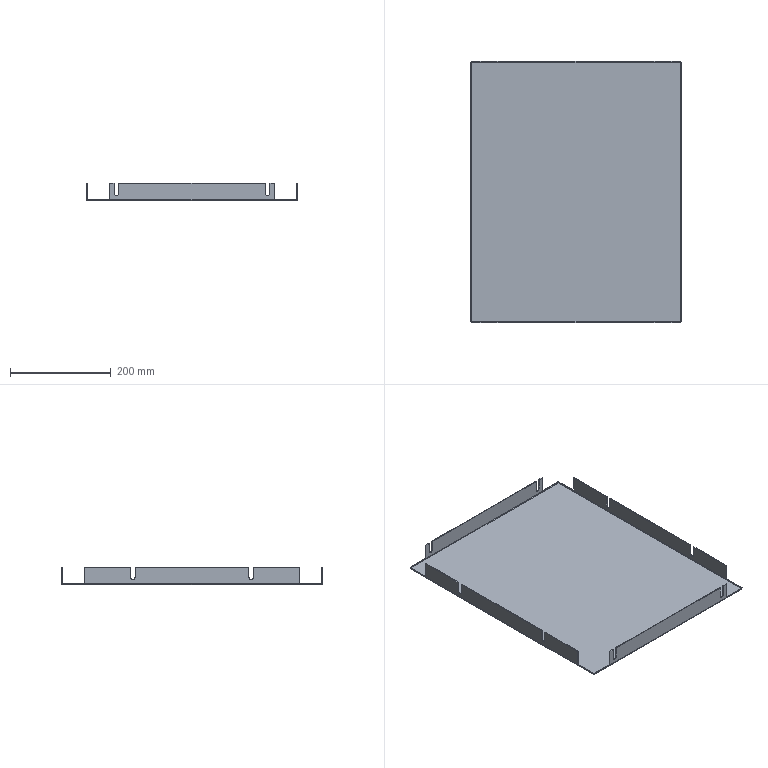Part | SolidWorks | features BaseBody 1 | 1 solid | 90 faces | box 418 x 518 x 35 mm | volume 397188 mm3 | plane 62 | cylinder 20 | spline 8 | commonest cylinder face diameters 9 x12 1.473 x4 4.473 x4